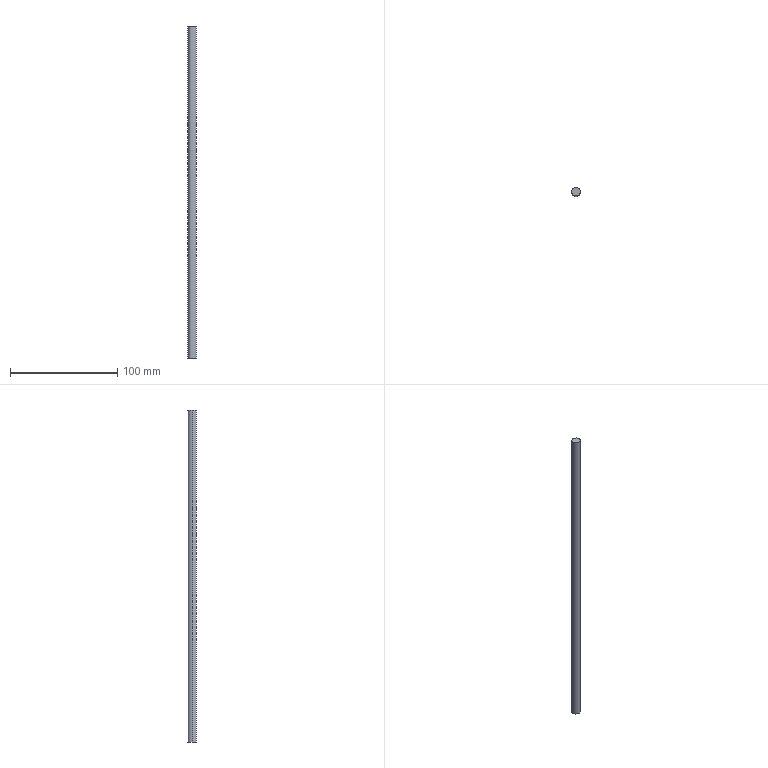Part | STEP file | 1 solid | 4 faces | box 8 x 8 x 310 mm | volume 15582 mm3 | cylinder 2 | plane 2 | commonest cylinder face diameters 8 x2
STEP:
#1=CARTESIAN_POINT('',(0.,0.,0.));
#2=DIRECTION('',(0.,0.,1.));
#3=DIRECTION('',(1.,0.,0.));
#4=AXIS2_PLACEMENT_3D('',#1,#2,#3);
#5=CARTESIAN_POINT('',(4.,0.,310.));
#6=VERTEX_POINT('',#5);
#7=CARTESIAN_POINT('',(-4.,0.,310.));
#8=VERTEX_POINT('',#7);
#9=CARTESIAN_POINT('',(0.,0.,310.));
#10=DIRECTION('',(0.,0.,1.));
#11=DIRECTION('',(1.,0.,0.));
#12=AXIS2_PLACEMENT_3D('',#9,#10,#11);
#13=CIRCLE('',#12,4.);
#14=CARTESIAN_POINT('',(0.,0.,310.));
#15=DIRECTION('',(0.,0.,-1.));
#16=DIRECTION('',(-1.,0.,0.));
#17=AXIS2_PLACEMENT_3D('',#14,#15,#16);
#18=CYLINDRICAL_SURFACE('',#17,4.);
#19=CARTESIAN_POINT('',(3.142,0.));
#20=DIRECTION('',(-1.,0.));
#21=VECTOR('',#20,1.);
#22=LINE('',#19,#21);
#23=(GEOMETRIC_REPRESENTATION_CONTEXT(2)PARAMETRIC_REPRESENTATION_CONTEXT()REPRESENTATION_CONTEXT('',''));
#24=DEFINITIONAL_REPRESENTATION('',(#22),#23);
#25=PCURVE('',#18,#24);
#26=CARTESIAN_POINT('',(0.,0.,310.));
#27=DIRECTION('',(0.,0.,1.));
#28=DIRECTION('',(1.,0.,0.));
#29=AXIS2_PLACEMENT_3D('',#26,#27,#28);
#30=PLANE('',#29);
#31=CARTESIAN_POINT('',(0.,0.));
#32=DIRECTION('',(1.,0.));
#33=AXIS2_PLACEMENT_2D('',#31,#32);
#34=CIRCLE('',#33,4.);
#35=(GEOMETRIC_REPRESENTATION_CONTEXT(2)PARAMETRIC_REPRESENTATION_CONTEXT()REPRESENTATION_CONTEXT('',''));
#36=DEFINITIONAL_REPRESENTATION('',(#34),#35);
#37=PCURVE('',#30,#36);
#38=SURFACE_CURVE('',#13,(#25,#37),.PCURVE_S1.);
#39=EDGE_CURVE('',#6,#8,#38,.T.);
#40=ORIENTED_EDGE('',*,*,#39,.F.);
#41=CARTESIAN_POINT('',(4.,0.,0.));
#42=VERTEX_POINT('',#41);
#43=CARTESIAN_POINT('',(4.,0.,310.));
#44=DIRECTION('',(0.,0.,-1.));
#45=VECTOR('',#44,1.);
#46=LINE('',#43,#45);
#47=CARTESIAN_POINT('',(3.142,0.));
#48=DIRECTION('',(0.,1.));
#49=VECTOR('',#48,1.);
#50=LINE('',#47,#49);
#51=(GEOMETRIC_REPRESENTATION_CONTEXT(2)PARAMETRIC_REPRESENTATION_CONTEXT()REPRESENTATION_CONTEXT('',''));
#52=DEFINITIONAL_REPRESENTATION('',(#50),#51);
#53=PCURVE('',#18,#52);
#54=CARTESIAN_POINT('',(0.,0.,310.));
#55=DIRECTION('',(0.,0.,-1.));
#56=DIRECTION('',(-1.,0.,0.));
#57=AXIS2_PLACEMENT_3D('',#54,#55,#56);
#58=CYLINDRICAL_SURFACE('',#57,4.);
#59=CARTESIAN_POINT('',(3.142,0.));
#60=DIRECTION('',(0.,1.));
#61=VECTOR('',#60,1.);
#62=LINE('',#59,#61);
#63=(GEOMETRIC_REPRESENTATION_CONTEXT(2)PARAMETRIC_REPRESENTATION_CONTEXT()REPRESENTATION_CONTEXT('',''));
#64=DEFINITIONAL_REPRESENTATION('',(#62),#63);
#65=PCURVE('',#58,#64);
#66=SURFACE_CURVE('',#46,(#53,#65),.PCURVE_S1.);
#67=EDGE_CURVE('',#6,#42,#66,.T.);
#68=ORIENTED_EDGE('',*,*,#67,.T.);
#69=CARTESIAN_POINT('',(-4.,0.,0.));
#70=VERTEX_POINT('',#69);
#71=CARTESIAN_POINT('',(0.,0.,0.));
#72=DIRECTION('',(0.,0.,1.));
#73=DIRECTION('',(1.,0.,0.));
#74=AXIS2_PLACEMENT_3D('',#71,#72,#73);
#75=CIRCLE('',#74,4.);
#76=CARTESIAN_POINT('',(3.142,310.));
#77=DIRECTION('',(-1.,0.));
#78=VECTOR('',#77,1.);
#79=LINE('',#76,#78);
#80=(GEOMETRIC_REPRESENTATION_CONTEXT(2)PARAMETRIC_REPRESENTATION_CONTEXT()REPRESENTATION_CONTEXT('',''));
#81=DEFINITIONAL_REPRESENTATION('',(#79),#80);
#82=PCURVE('',#18,#81);
#83=CARTESIAN_POINT('',(0.,0.,0.));
#84=DIRECTION('',(0.,0.,1.));
#85=DIRECTION('',(1.,0.,0.));
#86=AXIS2_PLACEMENT_3D('',#83,#84,#85);
#87=PLANE('',#86);
#88=CARTESIAN_POINT('',(0.,0.));
#89=DIRECTION('',(1.,0.));
#90=AXIS2_PLACEMENT_2D('',#88,#89);
#91=CIRCLE('',#90,4.);
#92=(GEOMETRIC_REPRESENTATION_CONTEXT(2)PARAMETRIC_REPRESENTATION_CONTEXT()REPRESENTATION_CONTEXT('',''));
#93=DEFINITIONAL_REPRESENTATION('',(#91),#92);
#94=PCURVE('',#87,#93);
#95=SURFACE_CURVE('',#75,(#82,#94),.PCURVE_S1.);
#96=EDGE_CURVE('',#42,#70,#95,.T.);
#97=ORIENTED_EDGE('',*,*,#96,.T.);
#98=CARTESIAN_POINT('',(-4.,0.,310.));
#99=DIRECTION('',(0.,0.,-1.));
#100=VECTOR('',#99,1.);
#101=LINE('',#98,#100);
#102=CARTESIAN_POINT('',(0.,0.));
#103=DIRECTION('',(0.,1.));
#104=VECTOR('',#103,1.);
#105=LINE('',#102,#104);
#106=(GEOMETRIC_REPRESENTATION_CONTEXT(2)PARAMETRIC_REPRESENTATION_CONTEXT()REPRESENTATION_CONTEXT('',''));
#107=DEFINITIONAL_REPRESENTATION('',(#105),#106);
#108=PCURVE('',#18,#107);
#109=CARTESIAN_POINT('',(6.283,0.));
#110=DIRECTION('',(0.,1.));
#111=VECTOR('',#110,1.);
#112=LINE('',#109,#111);
#113=(GEOMETRIC_REPRESENTATION_CONTEXT(2)PARAMETRIC_REPRESENTATION_CONTEXT()REPRESENTATION_CONTEXT('',''));
#114=DEFINITIONAL_REPRESENTATION('',(#112),#113);
#115=PCURVE('',#58,#114);
#116=SURFACE_CURVE('',#101,(#108,#115),.PCURVE_S1.);
#117=EDGE_CURVE('',#8,#70,#116,.T.);
#118=ORIENTED_EDGE('',*,*,#117,.F.);
#119=EDGE_LOOP('',(#40,#68,#97,#118));
#120=FACE_BOUND('',#119,.T.);
#121=ADVANCED_FACE('',(#120),#18,.T.);
#122=ORIENTED_EDGE('',*,*,#67,.F.);
#123=CARTESIAN_POINT('',(0.,0.,310.));
#124=DIRECTION('',(0.,0.,1.));
#125=DIRECTION('',(1.,0.,0.));
#126=AXIS2_PLACEMENT_3D('',#123,#124,#125);
#127=CIRCLE('',#126,4.);
#128=CARTESIAN_POINT('',(9.425,0.));
#129=DIRECTION('',(-1.,0.));
#130=VECTOR('',#129,1.);
#131=LINE('',#128,#130);
#132=(GEOMETRIC_REPRESENTATION_CONTEXT(2)PARAMETRIC_REPRESENTATION_CONTEXT()REPRESENTATION_CONTEXT('',''));
#133=DEFINITIONAL_REPRESENTATION('',(#131),#132);
#134=PCURVE('',#58,#133);
#135=CARTESIAN_POINT('',(0.,0.));
#136=DIRECTION('',(1.,0.));
#137=AXIS2_PLACEMENT_2D('',#135,#136);
#138=CIRCLE('',#137,4.);
#139=(GEOMETRIC_REPRESENTATION_CONTEXT(2)PARAMETRIC_REPRESENTATION_CONTEXT()REPRESENTATION_CONTEXT('',''));
#140=DEFINITIONAL_REPRESENTATION('',(#138),#139);
#141=PCURVE('',#30,#140);
#142=SURFACE_CURVE('',#127,(#134,#141),.PCURVE_S1.);
#143=EDGE_CURVE('',#8,#6,#142,.T.);
#144=ORIENTED_EDGE('',*,*,#143,.F.);
#145=ORIENTED_EDGE('',*,*,#117,.T.);
#146=CARTESIAN_POINT('',(0.,0.,0.));
#147=DIRECTION('',(0.,0.,1.));
#148=DIRECTION('',(1.,0.,0.));
#149=AXIS2_PLACEMENT_3D('',#146,#147,#148);
#150=CIRCLE('',#149,4.);
#151=CARTESIAN_POINT('',(9.425,310.));
#152=DIRECTION('',(-1.,0.));
#153=VECTOR('',#152,1.);
#154=LINE('',#151,#153);
#155=(GEOMETRIC_REPRESENTATION_CONTEXT(2)PARAMETRIC_REPRESENTATION_CONTEXT()REPRESENTATION_CONTEXT('',''));
#156=DEFINITIONAL_REPRESENTATION('',(#154),#155);
#157=PCURVE('',#58,#156);
#158=CARTESIAN_POINT('',(0.,0.));
#159=DIRECTION('',(1.,0.));
#160=AXIS2_PLACEMENT_2D('',#158,#159);
#161=CIRCLE('',#160,4.);
#162=(GEOMETRIC_REPRESENTATION_CONTEXT(2)PARAMETRIC_REPRESENTATION_CONTEXT()REPRESENTATION_CONTEXT('',''));
#163=DEFINITIONAL_REPRESENTATION('',(#161),#162);
#164=PCURVE('',#87,#163);
#165=SURFACE_CURVE('',#150,(#157,#164),.PCURVE_S1.);
#166=EDGE_CURVE('',#70,#42,#165,.T.);
#167=ORIENTED_EDGE('',*,*,#166,.T.);
#168=EDGE_LOOP('',(#122,#144,#145,#167));
#169=FACE_BOUND('',#168,.T.);
#170=ADVANCED_FACE('',(#169),#58,.T.);
#171=ORIENTED_EDGE('',*,*,#143,.T.);
#172=ORIENTED_EDGE('',*,*,#39,.T.);
#173=EDGE_LOOP('',(#171,#172));
#174=FACE_BOUND('',#173,.T.);
#175=ADVANCED_FACE('',(#174),#30,.T.);
#176=ORIENTED_EDGE('',*,*,#166,.F.);
#177=ORIENTED_EDGE('',*,*,#96,.F.);
#178=EDGE_LOOP('',(#176,#177));
#179=FACE_BOUND('',#178,.T.);
#180=ADVANCED_FACE('',(#179),#87,.F.);
#181=CLOSED_SHELL('',(#121,#170,#175,#180));
#182=MANIFOLD_SOLID_BREP('',#181);
#183=(LENGTH_UNIT()NAMED_UNIT(*)SI_UNIT(.MILLI.,.METRE.));
#184=UNCERTAINTY_MEASURE_WITH_UNIT(LENGTH_MEASURE(0.0000001),#183,'','');
#185=(NAMED_UNIT(*)PLANE_ANGLE_UNIT()SI_UNIT($,.RADIAN.));
#186=(NAMED_UNIT(*)SI_UNIT($,.STERADIAN.)SOLID_ANGLE_UNIT());
#187=(GEOMETRIC_REPRESENTATION_CONTEXT(3)GLOBAL_UNCERTAINTY_ASSIGNED_CONTEXT((#184))GLOBAL_UNIT_ASSIGNED_CONTEXT((#183,#185,#186))REPRESENTATION_CONTEXT('',''));
#188=ADVANCED_BREP_SHAPE_REPRESENTATION('',(#4,#182),#187);